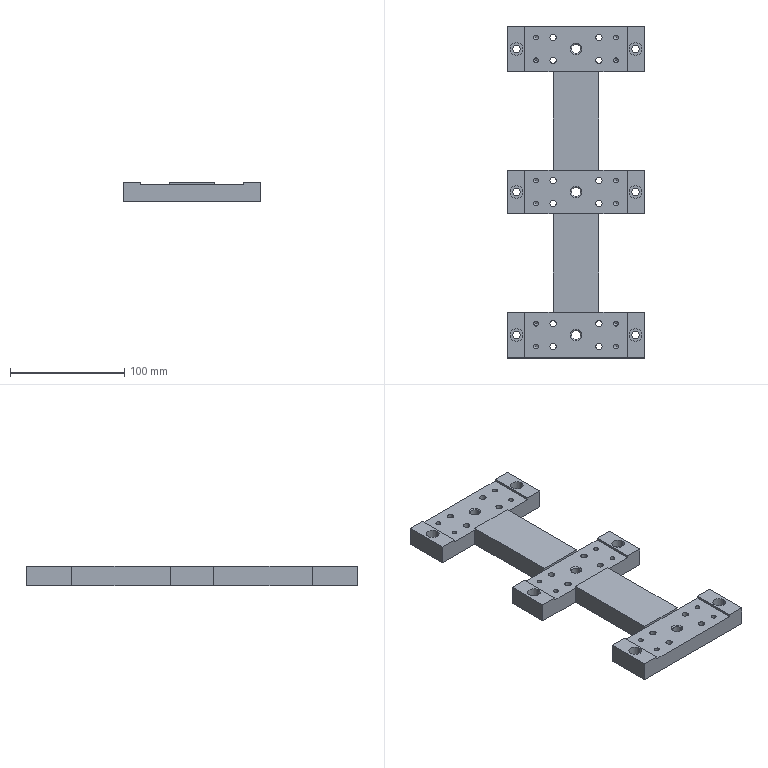Part | NX | features BREP 1 | 1 solid | 198 faces | box 120 x 290 x 17 mm | volume 318687 mm3 | cylinder 102 | plane 60 | cone 36 | commonest cylinder face diameters 4.2 x24 5.5 x24 9 x24 6.6 x12 11 x12 8 x6